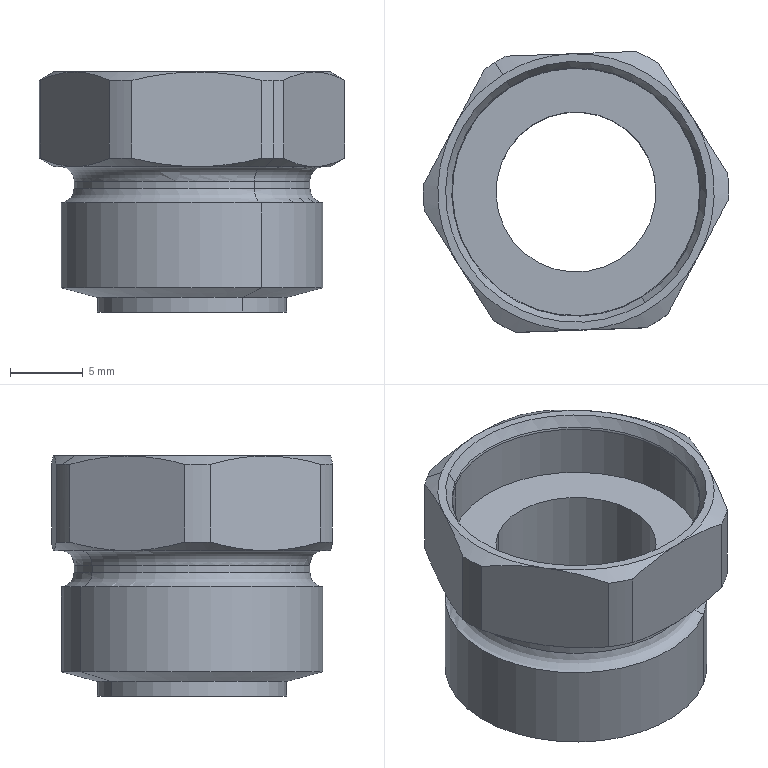Part | SolidWorks | features BaseBody 1 | 1 solid | 51 faces | box 21 x 19.305 x 16.5 mm | volume 2114 mm3 | cone 18 | cylinder 17 | plane 10 | torus 6 | commonest cylinder face diameters 21 x7 11 x2 13 x2 16.2 x2 17 x2 18 x2